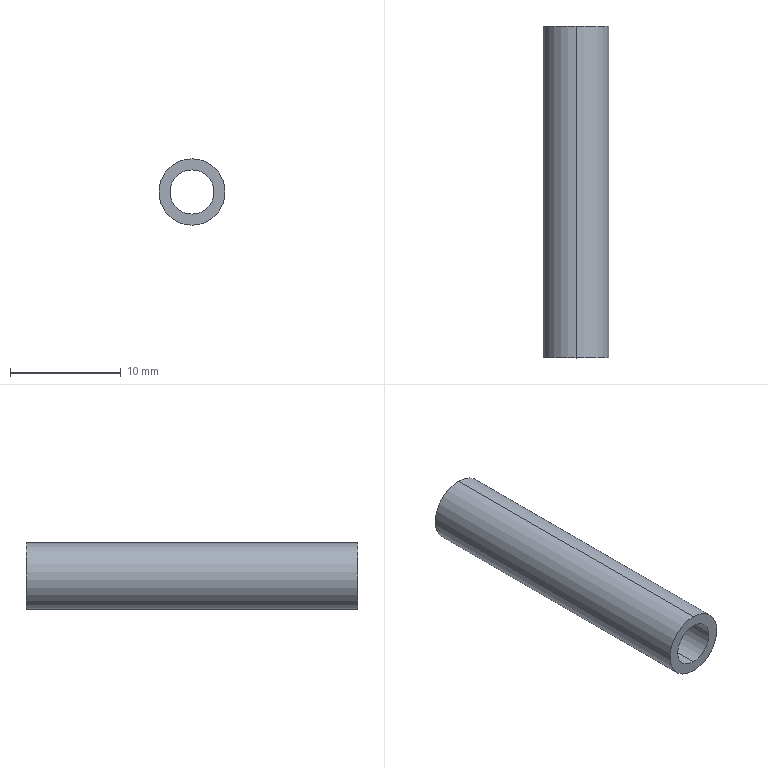Part | SolidWorks | features Extrusion 1 | 1 solid | 6 faces | box 6 x 30 x 6 mm | volume 471.239 mm3 | cylinder 4 | plane 2 | commonest cylinder face diameters 4 x2 6 x2
STEP:
#1=CARTESIAN_POINT('',(0.,30.,-2.));
#2=VERTEX_POINT('',#1);
#3=CARTESIAN_POINT('',(0.,30.,2.));
#4=VERTEX_POINT('',#3);
#5=CARTESIAN_POINT('',(0.,30.,0.));
#6=DIRECTION('',(0.,1.,0.));
#7=DIRECTION('',(0.,0.,1.));
#8=AXIS2_PLACEMENT_3D('',#5,#6,#7);
#9=CIRCLE('',#8,2.);
#10=EDGE_CURVE('',#2,#4,#9,.T.);
#11=ORIENTED_EDGE('',*,*,#10,.T.);
#12=CARTESIAN_POINT('',(0.,0.,2.));
#13=VERTEX_POINT('',#12);
#14=CARTESIAN_POINT('',(0.,30.,2.));
#15=DIRECTION('',(0.,-1.,0.));
#16=VECTOR('',#15,1000.);
#17=LINE('',#14,#16);
#18=EDGE_CURVE('',#4,#13,#17,.T.);
#19=ORIENTED_EDGE('',*,*,#18,.T.);
#20=CARTESIAN_POINT('',(0.,0.,-2.));
#21=VERTEX_POINT('',#20);
#22=CARTESIAN_POINT('',(0.,0.,0.));
#23=DIRECTION('',(0.,1.,0.));
#24=DIRECTION('',(0.,0.,1.));
#25=AXIS2_PLACEMENT_3D('',#22,#23,#24);
#26=CIRCLE('',#25,2.);
#27=EDGE_CURVE('',#21,#13,#26,.T.);
#28=ORIENTED_EDGE('',*,*,#27,.F.);
#29=CARTESIAN_POINT('',(0.,30.,-2.));
#30=DIRECTION('',(0.,-1.,0.));
#31=VECTOR('',#30,1000.);
#32=LINE('',#29,#31);
#33=EDGE_CURVE('',#2,#21,#32,.T.);
#34=ORIENTED_EDGE('',*,*,#33,.F.);
#35=EDGE_LOOP('',(#11,#19,#28,#34));
#36=FACE_OUTER_BOUND('',#35,.T.);
#37=CARTESIAN_POINT('',(0.,30.,0.));
#38=DIRECTION('',(0.,-1.,0.));
#39=DIRECTION('',(0.,0.,-1.));
#40=AXIS2_PLACEMENT_3D('',#37,#38,#39);
#41=CYLINDRICAL_SURFACE('',#40,2.);
#42=ADVANCED_FACE('',(#36),#41,.F.);
#43=CARTESIAN_POINT('',(0.,30.,3.));
#44=VERTEX_POINT('',#43);
#45=CARTESIAN_POINT('',(0.,30.,-3.));
#46=VERTEX_POINT('',#45);
#47=CARTESIAN_POINT('',(0.,30.,0.));
#48=DIRECTION('',(0.,1.,0.));
#49=DIRECTION('',(0.,0.,1.));
#50=AXIS2_PLACEMENT_3D('',#47,#48,#49);
#51=CIRCLE('',#50,3.);
#52=EDGE_CURVE('',#44,#46,#51,.T.);
#53=ORIENTED_EDGE('',*,*,#52,.F.);
#54=CARTESIAN_POINT('',(0.,0.,3.));
#55=VERTEX_POINT('',#54);
#56=CARTESIAN_POINT('',(0.,30.,3.));
#57=DIRECTION('',(0.,-1.,0.));
#58=VECTOR('',#57,1000.);
#59=LINE('',#56,#58);
#60=EDGE_CURVE('',#44,#55,#59,.T.);
#61=ORIENTED_EDGE('',*,*,#60,.T.);
#62=CARTESIAN_POINT('',(0.,0.,-3.));
#63=VERTEX_POINT('',#62);
#64=CARTESIAN_POINT('',(0.,0.,0.));
#65=DIRECTION('',(0.,1.,0.));
#66=DIRECTION('',(0.,0.,1.));
#67=AXIS2_PLACEMENT_3D('',#64,#65,#66);
#68=CIRCLE('',#67,3.);
#69=EDGE_CURVE('',#55,#63,#68,.T.);
#70=ORIENTED_EDGE('',*,*,#69,.T.);
#71=CARTESIAN_POINT('',(0.,30.,-3.));
#72=DIRECTION('',(0.,-1.,0.));
#73=VECTOR('',#72,1000.);
#74=LINE('',#71,#73);
#75=EDGE_CURVE('',#46,#63,#74,.T.);
#76=ORIENTED_EDGE('',*,*,#75,.F.);
#77=EDGE_LOOP('',(#53,#61,#70,#76));
#78=FACE_OUTER_BOUND('',#77,.T.);
#79=CARTESIAN_POINT('',(0.,30.,0.));
#80=DIRECTION('',(0.,-1.,0.));
#81=DIRECTION('',(0.,0.,-1.));
#82=AXIS2_PLACEMENT_3D('',#79,#80,#81);
#83=CYLINDRICAL_SURFACE('',#82,3.);
#84=ADVANCED_FACE('',(#78),#83,.T.);
#85=CARTESIAN_POINT('',(0.,30.,0.));
#86=DIRECTION('',(0.,1.,0.));
#87=DIRECTION('',(0.,0.,1.));
#88=AXIS2_PLACEMENT_3D('',#85,#86,#87);
#89=CIRCLE('',#88,3.);
#90=EDGE_CURVE('',#46,#44,#89,.T.);
#91=ORIENTED_EDGE('',*,*,#90,.T.);
#92=ORIENTED_EDGE('',*,*,#52,.T.);
#93=EDGE_LOOP('',(#91,#92));
#94=FACE_OUTER_BOUND('',#93,.T.);
#95=ORIENTED_EDGE('',*,*,#10,.F.);
#96=CARTESIAN_POINT('',(0.,30.,0.));
#97=DIRECTION('',(0.,1.,0.));
#98=DIRECTION('',(0.,0.,1.));
#99=AXIS2_PLACEMENT_3D('',#96,#97,#98);
#100=CIRCLE('',#99,2.);
#101=EDGE_CURVE('',#4,#2,#100,.T.);
#102=ORIENTED_EDGE('',*,*,#101,.F.);
#103=EDGE_LOOP('',(#95,#102));
#104=FACE_BOUND('',#103,.T.);
#105=CARTESIAN_POINT('',(0.,30.,0.));
#106=DIRECTION('',(0.,1.,0.));
#107=DIRECTION('',(0.,0.,1.));
#108=AXIS2_PLACEMENT_3D('',#105,#106,#107);
#109=PLANE('',#108);
#110=ADVANCED_FACE('',(#94,#104),#109,.T.);
#111=CARTESIAN_POINT('',(0.,0.,0.));
#112=DIRECTION('',(0.,1.,0.));
#113=DIRECTION('',(0.,0.,1.));
#114=AXIS2_PLACEMENT_3D('',#111,#112,#113);
#115=CIRCLE('',#114,3.);
#116=EDGE_CURVE('',#63,#55,#115,.T.);
#117=ORIENTED_EDGE('',*,*,#116,.F.);
#118=ORIENTED_EDGE('',*,*,#69,.F.);
#119=EDGE_LOOP('',(#117,#118));
#120=FACE_OUTER_BOUND('',#119,.T.);
#121=ORIENTED_EDGE('',*,*,#27,.T.);
#122=CARTESIAN_POINT('',(0.,0.,0.));
#123=DIRECTION('',(0.,1.,0.));
#124=DIRECTION('',(0.,0.,1.));
#125=AXIS2_PLACEMENT_3D('',#122,#123,#124);
#126=CIRCLE('',#125,2.);
#127=EDGE_CURVE('',#13,#21,#126,.T.);
#128=ORIENTED_EDGE('',*,*,#127,.T.);
#129=EDGE_LOOP('',(#121,#128));
#130=FACE_BOUND('',#129,.T.);
#131=CARTESIAN_POINT('',(0.,0.,0.));
#132=DIRECTION('',(0.,1.,0.));
#133=DIRECTION('',(0.,0.,1.));
#134=AXIS2_PLACEMENT_3D('',#131,#132,#133);
#135=PLANE('',#134);
#136=ADVANCED_FACE('',(#120,#130),#135,.F.);
#137=ORIENTED_EDGE('',*,*,#60,.F.);
#138=ORIENTED_EDGE('',*,*,#90,.F.);
#139=ORIENTED_EDGE('',*,*,#75,.T.);
#140=ORIENTED_EDGE('',*,*,#116,.T.);
#141=EDGE_LOOP('',(#137,#138,#139,#140));
#142=FACE_OUTER_BOUND('',#141,.T.);
#143=CARTESIAN_POINT('',(0.,30.,0.));
#144=DIRECTION('',(0.,-1.,0.));
#145=DIRECTION('',(0.,0.,-1.));
#146=AXIS2_PLACEMENT_3D('',#143,#144,#145);
#147=CYLINDRICAL_SURFACE('',#146,3.);
#148=ADVANCED_FACE('',(#142),#147,.T.);
#149=ORIENTED_EDGE('',*,*,#18,.F.);
#150=ORIENTED_EDGE('',*,*,#101,.T.);
#151=ORIENTED_EDGE('',*,*,#33,.T.);
#152=ORIENTED_EDGE('',*,*,#127,.F.);
#153=EDGE_LOOP('',(#149,#150,#151,#152));
#154=FACE_OUTER_BOUND('',#153,.T.);
#155=CARTESIAN_POINT('',(0.,30.,0.));
#156=DIRECTION('',(0.,-1.,0.));
#157=DIRECTION('',(0.,0.,-1.));
#158=AXIS2_PLACEMENT_3D('',#155,#156,#157);
#159=CYLINDRICAL_SURFACE('',#158,2.);
#160=ADVANCED_FACE('',(#154),#159,.F.);
#161=CLOSED_SHELL('',(#42,#84,#110,#136,#148,#160));
#162=MANIFOLD_SOLID_BREP('',#161);
#163=CARTESIAN_POINT('',(0.,0.,0.));
#164=DIRECTION('',(0.,0.,1.));
#165=DIRECTION('',(1.,0.,0.));
#166=AXIS2_PLACEMENT_3D('',#163,#164,#165);
#167=(LENGTH_UNIT()NAMED_UNIT(*)SI_UNIT(.MILLI.,.METRE.));
#168=UNCERTAINTY_MEASURE_WITH_UNIT(LENGTH_MEASURE(0.00001),#167,'','');
#169=(NAMED_UNIT(*)PLANE_ANGLE_UNIT()SI_UNIT($,.RADIAN.));
#170=(NAMED_UNIT(*)SI_UNIT($,.STERADIAN.)SOLID_ANGLE_UNIT());
#171=(GEOMETRIC_REPRESENTATION_CONTEXT(3)GLOBAL_UNCERTAINTY_ASSIGNED_CONTEXT((#168))GLOBAL_UNIT_ASSIGNED_CONTEXT((#167,#169,#170))REPRESENTATION_CONTEXT('',''));
#172=ADVANCED_BREP_SHAPE_REPRESENTATION('',(#162,#166),#171);